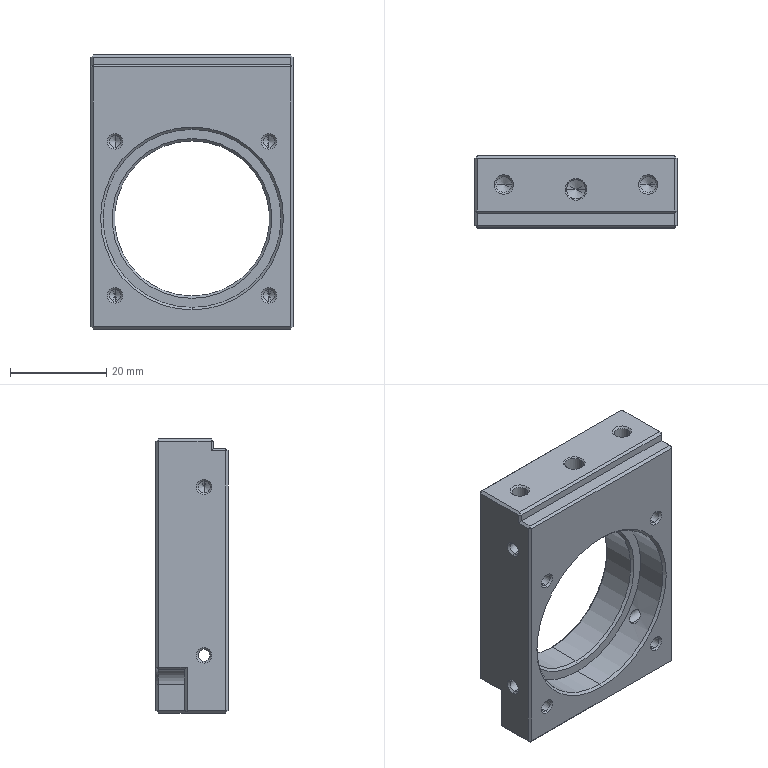Part | SolidWorks | features HoleWzd 6, ICE 4, Chamfer 1, Extrusion 1 | 1 solid | 146 faces | box 42 x 15 x 57 mm | volume 19915 mm3 | plane 58 | cone 56 | cylinder 32 | commonest cylinder face diameters 2.5 x16 2.05 x4 3.3 x4 4 x2 6 x2 32.2 x2